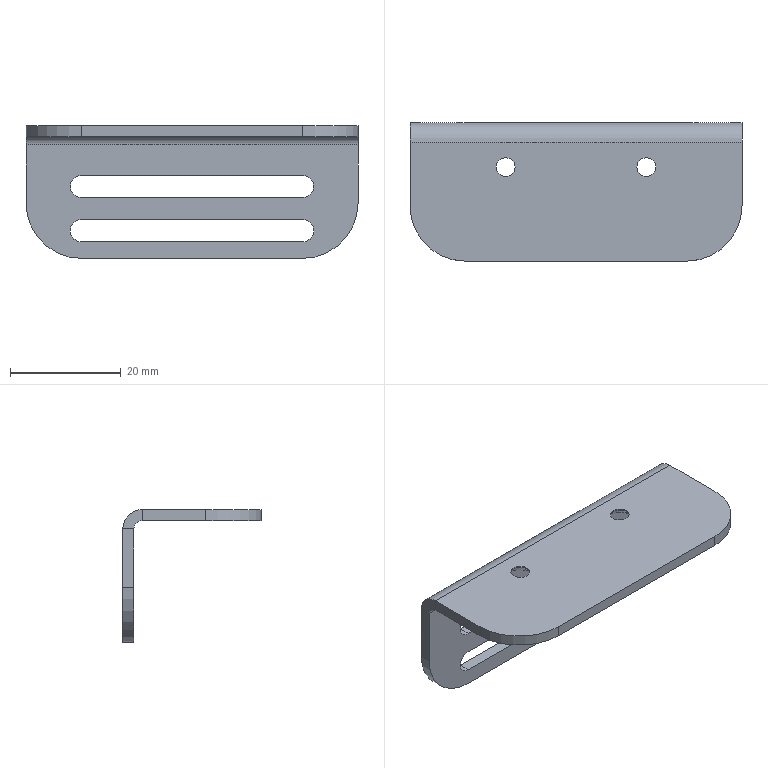Part | STEP file | BPSP-L-17 Pull Sensor Mounting Plate_Default | 1 solid | 34 faces | box 60 x 25 x 24 mm | volume 4566 mm3 | plane 16 | cylinder 14 | cone 4 | commonest cylinder face diameters 3.4 x4 4 x4 20 x4 3 x1 7 x1